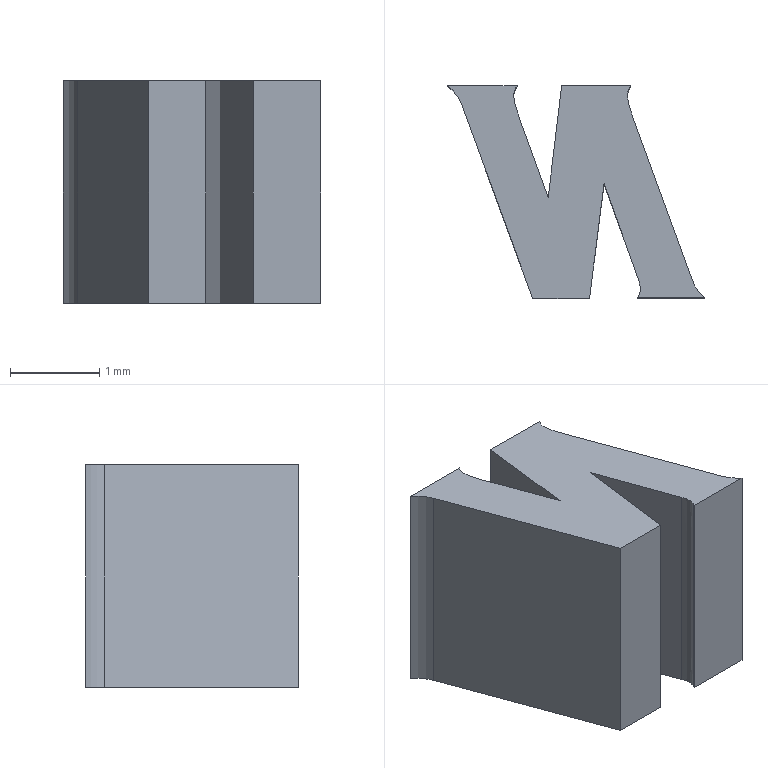Part | STEP file | lll_id1178_x_t | 1 solid | 18 faces | box 2.9 x 2.384 x 2.5 mm | volume 9.21 mm3 | plane 12 | other 4 | cylinder 2 | commonest cylinder face diameters 0.832 x1 0.919 x1
STEP:
#1=CARTESIAN_POINT('',(390.808,125.708,2.35));
#2=VERTEX_POINT('',#1);
#3=CARTESIAN_POINT('',(390.144,127.533,2.35));
#4=VERTEX_POINT('',#3);
#5=CARTESIAN_POINT('',(390.144,127.533,2.35));
#6=DIRECTION('',(-0.3422,0.9396,0.));
#7=VECTOR('',#6,1.);
#8=LINE('',#5,#7);
#9=EDGE_CURVE('',#2,#4,#8,.T.);
#10=ORIENTED_EDGE('',*,*,#9,.F.);
#11=CARTESIAN_POINT('',(390.808,125.708,-0.15));
#12=VERTEX_POINT('',#11);
#13=CARTESIAN_POINT('',(390.808,125.708,-0.15));
#14=DIRECTION('',(0.,0.,-1.));
#15=VECTOR('',#14,1.);
#16=LINE('',#13,#15);
#17=EDGE_CURVE('',#2,#12,#16,.T.);
#18=ORIENTED_EDGE('',*,*,#17,.T.);
#19=CARTESIAN_POINT('',(390.144,127.533,-0.15));
#20=VERTEX_POINT('',#19);
#21=CARTESIAN_POINT('',(390.144,127.533,-0.15));
#22=DIRECTION('',(-0.3422,0.9396,0.));
#23=VECTOR('',#22,1.);
#24=LINE('',#21,#23);
#25=EDGE_CURVE('',#12,#20,#24,.T.);
#26=ORIENTED_EDGE('',*,*,#25,.T.);
#27=CARTESIAN_POINT('',(390.144,127.533,-0.15));
#28=DIRECTION('',(0.,0.,-1.));
#29=VECTOR('',#28,1.);
#30=LINE('',#27,#29);
#31=EDGE_CURVE('',#4,#20,#30,.T.);
#32=ORIENTED_EDGE('',*,*,#31,.F.);
#33=EDGE_LOOP('',(#10,#18,#26,#32));
#34=FACE_OUTER_BOUND('',#33,.T.);
#35=CARTESIAN_POINT('',(390.144,127.533,-0.15));
#36=DIRECTION('',(-0.9396,-0.3422,0.));
#37=DIRECTION('',(-0.3422,0.9396,0.));
#38=AXIS2_PLACEMENT_3D('',#35,#36,#37);
#39=PLANE('',#38);
#40=ADVANCED_FACE('',(#34),#39,.F.);
#41=CARTESIAN_POINT('',(390.953,125.495,2.35));
#42=VERTEX_POINT('',#41);
#43=CARTESIAN_POINT('',(391.244,125.853,2.35));
#44=DIRECTION('',(0.,0.,-1.));
#45=DIRECTION('',(-1.,0.,0.));
#46=AXIS2_PLACEMENT_3D('',#43,#44,#45);
#47=CIRCLE('',#46,0.4594);
#48=EDGE_CURVE('',#42,#2,#47,.T.);
#49=ORIENTED_EDGE('',*,*,#48,.F.);
#50=CARTESIAN_POINT('',(390.953,125.495,-0.15));
#51=VERTEX_POINT('',#50);
#52=CARTESIAN_POINT('',(390.959,125.492,2.35));
#53=DIRECTION('',(0.,0.,-1.));
#54=VECTOR('',#53,1.);
#55=LINE('',#52,#54);
#56=EDGE_CURVE('',#42,#51,#55,.T.);
#57=ORIENTED_EDGE('',*,*,#56,.T.);
#58=CARTESIAN_POINT('',(391.244,125.853,-0.15));
#59=DIRECTION('',(0.,0.,-1.));
#60=DIRECTION('',(-1.,0.,0.));
#61=AXIS2_PLACEMENT_3D('',#58,#59,#60);
#62=CIRCLE('',#61,0.4594);
#63=EDGE_CURVE('',#51,#12,#62,.T.);
#64=ORIENTED_EDGE('',*,*,#63,.T.);
#65=ORIENTED_EDGE('',*,*,#17,.F.);
#66=EDGE_LOOP('',(#49,#57,#64,#65));
#67=FACE_OUTER_BOUND('',#66,.T.);
#68=CARTESIAN_POINT('',(391.244,125.853,-0.15));
#69=DIRECTION('',(0.,0.,1.));
#70=DIRECTION('',(1.,0.,0.));
#71=AXIS2_PLACEMENT_3D('',#68,#69,#70);
#72=CYLINDRICAL_SURFACE('',#71,0.4594);
#73=ADVANCED_FACE('',(#67),#72,.F.);
#74=CARTESIAN_POINT('',(390.2,125.495,2.35));
#75=VERTEX_POINT('',#74);
#76=CARTESIAN_POINT('',(390.953,125.492,2.35));
#77=DIRECTION('',(1.,0.,0.));
#78=VECTOR('',#77,1.);
#79=LINE('',#76,#78);
#80=EDGE_CURVE('',#75,#42,#79,.T.);
#81=ORIENTED_EDGE('',*,*,#80,.F.);
#82=CARTESIAN_POINT('',(390.2,125.495,-0.15));
#83=VERTEX_POINT('',#82);
#84=CARTESIAN_POINT('',(390.196,125.492,2.35));
#85=DIRECTION('',(0.,0.,-1.));
#86=VECTOR('',#85,1.);
#87=LINE('',#84,#86);
#88=EDGE_CURVE('',#75,#83,#87,.T.);
#89=ORIENTED_EDGE('',*,*,#88,.T.);
#90=CARTESIAN_POINT('',(390.953,125.492,-0.15));
#91=DIRECTION('',(1.,0.,0.));
#92=VECTOR('',#91,1.);
#93=LINE('',#90,#92);
#94=EDGE_CURVE('',#83,#51,#93,.T.);
#95=ORIENTED_EDGE('',*,*,#94,.T.);
#96=ORIENTED_EDGE('',*,*,#56,.F.);
#97=EDGE_LOOP('',(#81,#89,#95,#96));
#98=FACE_OUTER_BOUND('',#97,.T.);
#99=CARTESIAN_POINT('',(390.953,125.492,-0.15));
#100=DIRECTION('',(0.,1.,0.));
#101=DIRECTION('',(0.,0.,1.));
#102=AXIS2_PLACEMENT_3D('',#99,#100,#101);
#103=PLANE('',#102);
#104=ADVANCED_FACE('',(#98),#103,.F.);
#105=CARTESIAN_POINT('',(390.22,125.536,2.35));
#106=VERTEX_POINT('',#105);
#107=CARTESIAN_POINT('',(390.22,125.536,2.35));
#108=CARTESIAN_POINT('',(390.215,125.523,2.35));
#109=CARTESIAN_POINT('',(390.208,125.51,2.35));
#110=CARTESIAN_POINT('',(390.199,125.498,2.35));
#111=(BOUNDED_CURVE()B_SPLINE_CURVE(3,(#107,#108,#109,#110),.UNSPECIFIED.,.F.,.F.)B_SPLINE_CURVE_WITH_KNOTS((4,4),(0.,1.),.UNSPECIFIED.)CURVE()GEOMETRIC_REPRESENTATION_ITEM()RATIONAL_B_SPLINE_CURVE((0.5015,0.4995,0.4995,0.5015))REPRESENTATION_ITEM(''));
#112=EDGE_CURVE('',#106,#75,#111,.T.);
#113=ORIENTED_EDGE('',*,*,#112,.F.);
#114=CARTESIAN_POINT('',(390.22,125.536,-0.15));
#115=VERTEX_POINT('',#114);
#116=CARTESIAN_POINT('',(390.22,125.536,-0.15));
#117=DIRECTION('',(0.,0.,-1.));
#118=VECTOR('',#117,1.);
#119=LINE('',#116,#118);
#120=EDGE_CURVE('',#106,#115,#119,.T.);
#121=ORIENTED_EDGE('',*,*,#120,.T.);
#122=CARTESIAN_POINT('',(390.22,125.536,-0.15));
#123=CARTESIAN_POINT('',(390.215,125.523,-0.15));
#124=CARTESIAN_POINT('',(390.208,125.51,-0.15));
#125=CARTESIAN_POINT('',(390.199,125.497,-0.15));
#126=CARTESIAN_POINT('',(390.199,125.496,-0.15));
#127=CARTESIAN_POINT('',(390.198,125.496,-0.15));
#128=(BOUNDED_CURVE()B_SPLINE_CURVE(3,(#122,#123,#124,#125,#126,#127),.UNSPECIFIED.,.F.,.F.)B_SPLINE_CURVE_WITH_KNOTS((4,2,4),(0.,0.9573,1.),.UNSPECIFIED.)CURVE()GEOMETRIC_REPRESENTATION_ITEM()RATIONAL_B_SPLINE_CURVE((0.5015,0.4995,0.4995,0.5015,0.5015,0.5015))REPRESENTATION_ITEM(''));
#129=EDGE_CURVE('',#115,#83,#128,.T.);
#130=ORIENTED_EDGE('',*,*,#129,.T.);
#131=ORIENTED_EDGE('',*,*,#88,.F.);
#132=EDGE_LOOP('',(#113,#121,#130,#131));
#133=FACE_OUTER_BOUND('',#132,.T.);
#134=CARTESIAN_POINT('',(390.196,125.492,-0.15));
#135=CARTESIAN_POINT('',(390.196,125.493,-0.15));
#136=CARTESIAN_POINT('',(390.197,125.494,-0.15));
#137=CARTESIAN_POINT('',(390.198,125.495,-0.15));
#138=CARTESIAN_POINT('',(390.198,125.495,-0.15));
#139=CARTESIAN_POINT('',(390.199,125.496,-0.15));
#140=CARTESIAN_POINT('',(390.199,125.497,-0.15));
#141=CARTESIAN_POINT('',(390.208,125.51,-0.15));
#142=CARTESIAN_POINT('',(390.215,125.523,-0.15));
#143=CARTESIAN_POINT('',(390.22,125.536,-0.15));
#144=(BOUNDED_CURVE()B_SPLINE_CURVE(3,(#134,#135,#136,#137,#138,#139,#140,#141,#142,#143),.UNSPECIFIED.,.F.,.F.)B_SPLINE_CURVE_WITH_KNOTS((4,2,2,2,4),(0.,0.04179,0.08327,0.1224,1.),.UNSPECIFIED.)CURVE()GEOMETRIC_REPRESENTATION_ITEM()RATIONAL_B_SPLINE_CURVE((0.5015,0.5015,0.5015,0.5015,0.5015,0.5015,0.5015,0.4995,0.4995,0.5015))REPRESENTATION_ITEM(''));
#145=DIRECTION('',(0.,0.,1.));
#146=VECTOR('',#145,1.);
#147=SURFACE_OF_LINEAR_EXTRUSION('',#144,#146);
#148=ADVANCED_FACE('',(#133),#147,.F.);
#149=CARTESIAN_POINT('',(390.211,125.704,2.35));
#150=VERTEX_POINT('',#149);
#151=CARTESIAN_POINT('',(390.211,125.704,2.35));
#152=CARTESIAN_POINT('',(390.214,125.693,2.35));
#153=CARTESIAN_POINT('',(390.218,125.683,2.35));
#154=CARTESIAN_POINT('',(390.224,125.661,2.35));
#155=CARTESIAN_POINT('',(390.226,125.65,2.35));
#156=CARTESIAN_POINT('',(390.23,125.628,2.35));
#157=CARTESIAN_POINT('',(390.231,125.617,2.35));
#158=CARTESIAN_POINT('',(390.232,125.599,2.35));
#159=CARTESIAN_POINT('',(390.232,125.592,2.35));
#160=CARTESIAN_POINT('',(390.23,125.568,2.35));
#161=CARTESIAN_POINT('',(390.226,125.552,2.35));
#162=CARTESIAN_POINT('',(390.22,125.536,2.35));
#163=(BOUNDED_CURVE()B_SPLINE_CURVE(3,(#151,#152,#153,#154,#155,#156,#157,#158,#159,#160,#161,#162),.UNSPECIFIED.,.F.,.F.)B_SPLINE_CURVE_WITH_KNOTS((4,2,2,2,2,4),(0.,0.1952,0.3909,0.5862,0.7038,1.),.UNSPECIFIED.)CURVE()GEOMETRIC_REPRESENTATION_ITEM()RATIONAL_B_SPLINE_CURVE((0.5015,0.5013,0.5013,0.5011,0.5011,0.5008,0.5008,0.5011,0.5011,0.4975,0.4975,0.5015))REPRESENTATION_ITEM(''));
#164=EDGE_CURVE('',#150,#106,#163,.T.);
#165=ORIENTED_EDGE('',*,*,#164,.F.);
#166=CARTESIAN_POINT('',(390.211,125.704,-0.15));
#167=VERTEX_POINT('',#166);
#168=CARTESIAN_POINT('',(390.211,125.704,-0.15));
#169=DIRECTION('',(0.,0.,-1.));
#170=VECTOR('',#169,1.);
#171=LINE('',#168,#170);
#172=EDGE_CURVE('',#150,#167,#171,.T.);
#173=ORIENTED_EDGE('',*,*,#172,.T.);
#174=CARTESIAN_POINT('',(390.211,125.704,-0.15));
#175=CARTESIAN_POINT('',(390.214,125.693,-0.15));
#176=CARTESIAN_POINT('',(390.218,125.683,-0.15));
#177=CARTESIAN_POINT('',(390.224,125.661,-0.15));
#178=CARTESIAN_POINT('',(390.226,125.65,-0.15));
#179=CARTESIAN_POINT('',(390.23,125.628,-0.15));
#180=CARTESIAN_POINT('',(390.231,125.617,-0.15));
#181=CARTESIAN_POINT('',(390.232,125.599,-0.15));
#182=CARTESIAN_POINT('',(390.232,125.592,-0.15));
#183=CARTESIAN_POINT('',(390.23,125.568,-0.15));
#184=CARTESIAN_POINT('',(390.226,125.552,-0.15));
#185=CARTESIAN_POINT('',(390.22,125.536,-0.15));
#186=(BOUNDED_CURVE()B_SPLINE_CURVE(3,(#174,#175,#176,#177,#178,#179,#180,#181,#182,#183,#184,#185),.UNSPECIFIED.,.F.,.F.)B_SPLINE_CURVE_WITH_KNOTS((4,2,2,2,2,4),(0.,0.1952,0.3909,0.5862,0.7038,1.),.UNSPECIFIED.)CURVE()GEOMETRIC_REPRESENTATION_ITEM()RATIONAL_B_SPLINE_CURVE((0.5015,0.5013,0.5013,0.5011,0.5011,0.5008,0.5008,0.5011,0.5011,0.4975,0.4975,0.5015))REPRESENTATION_ITEM(''));
#187=EDGE_CURVE('',#167,#115,#186,.T.);
#188=ORIENTED_EDGE('',*,*,#187,.T.);
#189=ORIENTED_EDGE('',*,*,#120,.F.);
#190=EDGE_LOOP('',(#165,#173,#188,#189));
#191=FACE_OUTER_BOUND('',#190,.T.);
#192=CARTESIAN_POINT('',(390.22,125.536,-0.15));
#193=CARTESIAN_POINT('',(390.226,125.552,-0.15));
#194=CARTESIAN_POINT('',(390.23,125.568,-0.15));
#195=CARTESIAN_POINT('',(390.232,125.592,-0.15));
#196=CARTESIAN_POINT('',(390.232,125.599,-0.15));
#197=CARTESIAN_POINT('',(390.231,125.617,-0.15));
#198=CARTESIAN_POINT('',(390.23,125.628,-0.15));
#199=CARTESIAN_POINT('',(390.226,125.65,-0.15));
#200=CARTESIAN_POINT('',(390.224,125.661,-0.15));
#201=CARTESIAN_POINT('',(390.218,125.683,-0.15));
#202=CARTESIAN_POINT('',(390.214,125.693,-0.15));
#203=CARTESIAN_POINT('',(390.211,125.704,-0.15));
#204=(BOUNDED_CURVE()B_SPLINE_CURVE(3,(#192,#193,#194,#195,#196,#197,#198,#199,#200,#201,#202,#203),.UNSPECIFIED.,.F.,.F.)B_SPLINE_CURVE_WITH_KNOTS((4,2,2,2,2,4),(0.,0.2962,0.4138,0.6091,0.8048,1.),.UNSPECIFIED.)CURVE()GEOMETRIC_REPRESENTATION_ITEM()RATIONAL_B_SPLINE_CURVE((0.5015,0.4975,0.4975,0.5011,0.5011,0.5008,0.5008,0.5011,0.5011,0.5013,0.5013,0.5015))REPRESENTATION_ITEM(''));
#205=DIRECTION('',(0.,0.,1.));
#206=VECTOR('',#205,1.);
#207=SURFACE_OF_LINEAR_EXTRUSION('',#204,#206);
#208=ADVANCED_FACE('',(#191),#207,.F.);
#209=CARTESIAN_POINT('',(389.825,126.775,2.35));
#210=VERTEX_POINT('',#209);
#211=CARTESIAN_POINT('',(390.211,125.704,2.35));
#212=DIRECTION('',(0.3387,-0.9409,0.));
#213=VECTOR('',#212,1.);
#214=LINE('',#211,#213);
#215=EDGE_CURVE('',#210,#150,#214,.T.);
#216=ORIENTED_EDGE('',*,*,#215,.F.);
#217=CARTESIAN_POINT('',(389.825,126.775,-0.15));
#218=VERTEX_POINT('',#217);
#219=CARTESIAN_POINT('',(389.825,126.775,-0.15));
#220=DIRECTION('',(0.,0.,-1.));
#221=VECTOR('',#220,1.);
#222=LINE('',#219,#221);
#223=EDGE_CURVE('',#210,#218,#222,.T.);
#224=ORIENTED_EDGE('',*,*,#223,.T.);
#225=CARTESIAN_POINT('',(390.211,125.704,-0.15));
#226=DIRECTION('',(0.3387,-0.9409,0.));
#227=VECTOR('',#226,1.);
#228=LINE('',#225,#227);
#229=EDGE_CURVE('',#218,#167,#228,.T.);
#230=ORIENTED_EDGE('',*,*,#229,.T.);
#231=ORIENTED_EDGE('',*,*,#172,.F.);
#232=EDGE_LOOP('',(#216,#224,#230,#231));
#233=FACE_OUTER_BOUND('',#232,.T.);
#234=CARTESIAN_POINT('',(390.211,125.704,-0.15));
#235=DIRECTION('',(0.9409,0.3387,0.));
#236=DIRECTION('',(0.3387,-0.9409,0.));
#237=AXIS2_PLACEMENT_3D('',#234,#235,#236);
#238=PLANE('',#237);
#239=ADVANCED_FACE('',(#233),#238,.F.);
#240=CARTESIAN_POINT('',(389.662,125.492,2.35));
#241=VERTEX_POINT('',#240);
#242=CARTESIAN_POINT('',(389.825,126.775,2.35));
#243=DIRECTION('',(0.1257,0.9921,0.));
#244=VECTOR('',#243,1.);
#245=LINE('',#242,#244);
#246=EDGE_CURVE('',#241,#210,#245,.T.);
#247=ORIENTED_EDGE('',*,*,#246,.F.);
#248=CARTESIAN_POINT('',(389.662,125.492,-0.15));
#249=VERTEX_POINT('',#248);
#250=CARTESIAN_POINT('',(389.662,125.492,-0.15));
#251=DIRECTION('',(0.,0.,-1.));
#252=VECTOR('',#251,1.);
#253=LINE('',#250,#252);
#254=EDGE_CURVE('',#241,#249,#253,.T.);
#255=ORIENTED_EDGE('',*,*,#254,.T.);
#256=CARTESIAN_POINT('',(389.825,126.775,-0.15));
#257=DIRECTION('',(0.1257,0.9921,0.));
#258=VECTOR('',#257,1.);
#259=LINE('',#256,#258);
#260=EDGE_CURVE('',#249,#218,#259,.T.);
#261=ORIENTED_EDGE('',*,*,#260,.T.);
#262=ORIENTED_EDGE('',*,*,#223,.F.);
#263=EDGE_LOOP('',(#247,#255,#261,#262));
#264=FACE_OUTER_BOUND('',#263,.T.);
#265=CARTESIAN_POINT('',(389.825,126.775,-0.15));
#266=DIRECTION('',(-0.9921,0.1257,0.));
#267=DIRECTION('',(0.1257,0.9921,0.));
#268=AXIS2_PLACEMENT_3D('',#265,#266,#267);
#269=PLANE('',#268);
#270=ADVANCED_FACE('',(#264),#269,.F.);
#271=CARTESIAN_POINT('',(389.024,125.492,2.35));
#272=VERTEX_POINT('',#271);
#273=CARTESIAN_POINT('',(389.662,125.492,2.35));
#274=DIRECTION('',(1.,0.,0.));
#275=VECTOR('',#274,1.);
#276=LINE('',#273,#275);
#277=EDGE_CURVE('',#272,#241,#276,.T.);
#278=ORIENTED_EDGE('',*,*,#277,.F.);
#279=CARTESIAN_POINT('',(389.024,125.492,-0.15));
#280=VERTEX_POINT('',#279);
#281=CARTESIAN_POINT('',(389.024,125.492,-0.15));
#282=DIRECTION('',(0.,0.,-1.));
#283=VECTOR('',#282,1.);
#284=LINE('',#281,#283);
#285=EDGE_CURVE('',#272,#280,#284,.T.);
#286=ORIENTED_EDGE('',*,*,#285,.T.);
#287=CARTESIAN_POINT('',(389.662,125.492,-0.15));
#288=DIRECTION('',(1.,0.,0.));
#289=VECTOR('',#288,1.);
#290=LINE('',#287,#289);
#291=EDGE_CURVE('',#280,#249,#290,.T.);
#292=ORIENTED_EDGE('',*,*,#291,.T.);
#293=ORIENTED_EDGE('',*,*,#254,.F.);
#294=EDGE_LOOP('',(#278,#286,#292,#293));
#295=FACE_OUTER_BOUND('',#294,.T.);
#296=CARTESIAN_POINT('',(389.662,125.492,-0.15));
#297=DIRECTION('',(0.,1.,0.));
#298=DIRECTION('',(0.,0.,1.));
#299=AXIS2_PLACEMENT_3D('',#296,#297,#298);
#300=PLANE('',#299);
#301=ADVANCED_FACE('',(#295),#300,.F.);
#302=CARTESIAN_POINT('',(388.229,127.665,2.35));
#303=VERTEX_POINT('',#302);
#304=CARTESIAN_POINT('',(389.024,125.492,2.35));
#305=DIRECTION('',(0.3436,-0.9391,0.));
#306=VECTOR('',#305,1.);
#307=LINE('',#304,#306);
#308=EDGE_CURVE('',#303,#272,#307,.T.);
#309=ORIENTED_EDGE('',*,*,#308,.F.);
#310=CARTESIAN_POINT('',(388.229,127.665,-0.15));
#311=VERTEX_POINT('',#310);
#312=CARTESIAN_POINT('',(388.229,127.665,-0.15));
#313=DIRECTION('',(0.,0.,-1.));
#314=VECTOR('',#313,1.);
#315=LINE('',#312,#314);
#316=EDGE_CURVE('',#303,#311,#315,.T.);
#317=ORIENTED_EDGE('',*,*,#316,.T.);
#318=CARTESIAN_POINT('',(389.024,125.492,-0.15));
#319=DIRECTION('',(0.3436,-0.9391,0.));
#320=VECTOR('',#319,1.);
#321=LINE('',#318,#320);
#322=EDGE_CURVE('',#311,#280,#321,.T.);
#323=ORIENTED_EDGE('',*,*,#322,.T.);
#324=ORIENTED_EDGE('',*,*,#285,.F.);
#325=EDGE_LOOP('',(#309,#317,#323,#324));
#326=FACE_OUTER_BOUND('',#325,.T.);
#327=CARTESIAN_POINT('',(389.024,125.492,-0.15));
#328=DIRECTION('',(0.9391,0.3436,0.));
#329=DIRECTION('',(0.3436,-0.9391,0.));
#330=AXIS2_PLACEMENT_3D('',#327,#328,#329);
#331=PLANE('',#330);
#332=ADVANCED_FACE('',(#326),#331,.F.);
#333=CARTESIAN_POINT('',(388.068,127.874,2.35));
#334=VERTEX_POINT('',#333);
#335=CARTESIAN_POINT('',(387.837,127.525,2.35));
#336=DIRECTION('',(0.,0.,-1.));
#337=DIRECTION('',(-1.,0.,0.));
#338=AXIS2_PLACEMENT_3D('',#335,#336,#337);
#339=CIRCLE('',#338,0.4162);
#340=EDGE_CURVE('',#334,#303,#339,.T.);
#341=ORIENTED_EDGE('',*,*,#340,.F.);
#342=CARTESIAN_POINT('',(388.068,127.874,-0.15));
#343=VERTEX_POINT('',#342);
#344=CARTESIAN_POINT('',(388.059,127.877,2.35));
#345=DIRECTION('',(0.,0.,-1.));
#346=VECTOR('',#345,1.);
#347=LINE('',#344,#346);
#348=EDGE_CURVE('',#334,#343,#347,.T.);
#349=ORIENTED_EDGE('',*,*,#348,.T.);
#350=CARTESIAN_POINT('',(387.837,127.525,-0.15));
#351=DIRECTION('',(0.,0.,-1.));
#352=DIRECTION('',(-1.,0.,0.));
#353=AXIS2_PLACEMENT_3D('',#350,#351,#352);
#354=CIRCLE('',#353,0.4162);
#355=EDGE_CURVE('',#343,#311,#354,.T.);
#356=ORIENTED_EDGE('',*,*,#355,.T.);
#357=ORIENTED_EDGE('',*,*,#316,.F.);
#358=EDGE_LOOP('',(#341,#349,#356,#357));
#359=FACE_OUTER_BOUND('',#358,.T.);
#360=CARTESIAN_POINT('',(387.837,127.525,-0.15));
#361=DIRECTION('',(0.,0.,1.));
#362=DIRECTION('',(1.,0.,0.));
#363=AXIS2_PLACEMENT_3D('',#360,#361,#362);
#364=CYLINDRICAL_SURFACE('',#363,0.4162);
#365=ADVANCED_FACE('',(#359),#364,.F.);
#366=CARTESIAN_POINT('',(388.851,127.874,2.35));
#367=VERTEX_POINT('',#366);
#368=CARTESIAN_POINT('',(388.068,127.877,2.35));
#369=DIRECTION('',(-1.,0.,0.));
#370=VECTOR('',#369,1.);
#371=LINE('',#368,#370);
#372=EDGE_CURVE('',#367,#334,#371,.T.);
#373=ORIENTED_EDGE('',*,*,#372,.F.);
#374=CARTESIAN_POINT('',(388.851,127.874,-0.15));
#375=VERTEX_POINT('',#374);
#376=CARTESIAN_POINT('',(388.855,127.877,2.35));
#377=DIRECTION('',(0.,0.,-1.));
#378=VECTOR('',#377,1.);
#379=LINE('',#376,#378);
#380=EDGE_CURVE('',#367,#375,#379,.T.);
#381=ORIENTED_EDGE('',*,*,#380,.T.);
#382=CARTESIAN_POINT('',(388.068,127.877,-0.15));
#383=DIRECTION('',(-1.,0.,0.));
#384=VECTOR('',#383,1.);
#385=LINE('',#382,#384);
#386=EDGE_CURVE('',#375,#343,#385,.T.);
#387=ORIENTED_EDGE('',*,*,#386,.T.);
#388=ORIENTED_EDGE('',*,*,#348,.F.);
#389=EDGE_LOOP('',(#373,#381,#387,#388));
#390=FACE_OUTER_BOUND('',#389,.T.);
#391=CARTESIAN_POINT('',(388.068,127.877,-0.15));
#392=DIRECTION('',(0.,-1.,0.));
#393=DIRECTION('',(0.,0.,-1.));
#394=AXIS2_PLACEMENT_3D('',#391,#392,#393);
#395=PLANE('',#394);
#396=ADVANCED_FACE('',(#390),#395,.F.);
#397=CARTESIAN_POINT('',(388.868,127.533,2.35));
#398=VERTEX_POINT('',#397);
#399=CARTESIAN_POINT('',(388.868,127.533,2.35));
#400=CARTESIAN_POINT('',(388.86,127.554,2.35));
#401=CARTESIAN_POINT('',(388.853,127.575,2.35));
#402=CARTESIAN_POINT('',(388.841,127.614,2.35));
#403=CARTESIAN_POINT('',(388.836,127.631,2.35));
#404=CARTESIAN_POINT('',(388.827,127.66,2.35));
#405=CARTESIAN_POINT('',(388.825,127.671,2.35));
#406=CARTESIAN_POINT('',(388.819,127.692,2.35));
#407=CARTESIAN_POINT('',(388.817,127.703,2.35));
#408=CARTESIAN_POINT('',(388.814,127.723,2.35));
#409=CARTESIAN_POINT('',(388.813,127.733,2.35));
#410=CARTESIAN_POINT('',(388.811,127.755,2.35));
#411=CARTESIAN_POINT('',(388.811,127.768,2.35));
#412=CARTESIAN_POINT('',(388.815,127.81,2.35));
#413=CARTESIAN_POINT('',(388.826,127.839,2.35));
#414=CARTESIAN_POINT('',(388.846,127.865,2.35));
#415=CARTESIAN_POINT('',(388.849,127.868,2.35));
#416=CARTESIAN_POINT('',(388.851,127.871,2.35));
#417=(BOUNDED_CURVE()B_SPLINE_CURVE(3,(#399,#400,#401,#402,#403,#404,#405,#406,#407,#408,#409,#410,#411,#412,#413,#414,#415,#416),.UNSPECIFIED.,.F.,.F.)B_SPLINE_CURVE_WITH_KNOTS((4,2,2,2,2,2,2,2,4),(0.,0.1864,0.3417,0.4351,0.5283,0.6059,0.715,0.9678,1.),.UNSPECIFIED.)CURVE()GEOMETRIC_REPRESENTATION_ITEM()RATIONAL_B_SPLINE_CURVE((0.5001,0.5,0.5,0.5,0.5,0.5,0.5,0.4998,0.4998,0.4998,0.4998,0.4988,0.4988,0.4872,0.4872,0.5,0.5,0.5001))REPRESENTATION_ITEM(''));
#418=EDGE_CURVE('',#398,#367,#417,.T.);
#419=ORIENTED_EDGE('',*,*,#418,.F.);
#420=CARTESIAN_POINT('',(388.868,127.533,-0.15));
#421=VERTEX_POINT('',#420);
#422=CARTESIAN_POINT('',(388.868,127.533,-0.15));
#423=DIRECTION('',(0.,0.,-1.));
#424=VECTOR('',#423,1.);
#425=LINE('',#422,#424);
#426=EDGE_CURVE('',#398,#421,#425,.T.);
#427=ORIENTED_EDGE('',*,*,#426,.T.);
#428=CARTESIAN_POINT('',(388.868,127.533,-0.15));
#429=CARTESIAN_POINT('',(388.86,127.554,-0.15));
#430=CARTESIAN_POINT('',(388.853,127.575,-0.15));
#431=CARTESIAN_POINT('',(388.841,127.614,-0.15));
#432=CARTESIAN_POINT('',(388.836,127.631,-0.15));
#433=CARTESIAN_POINT('',(388.827,127.66,-0.15));
#434=CARTESIAN_POINT('',(388.825,127.671,-0.15));
#435=CARTESIAN_POINT('',(388.819,127.692,-0.15));
#436=CARTESIAN_POINT('',(388.817,127.703,-0.15));
#437=CARTESIAN_POINT('',(388.814,127.723,-0.15));
#438=CARTESIAN_POINT('',(388.813,127.733,-0.15));
#439=CARTESIAN_POINT('',(388.811,127.755,-0.15));
#440=CARTESIAN_POINT('',(388.811,127.768,-0.15));
#441=CARTESIAN_POINT('',(388.815,127.81,-0.15));
#442=CARTESIAN_POINT('',(388.826,127.839,-0.15));
#443=CARTESIAN_POINT('',(388.846,127.865,-0.15));
#444=CARTESIAN_POINT('',(388.849,127.868,-0.15));
#445=CARTESIAN_POINT('',(388.852,127.872,-0.15));
#446=CARTESIAN_POINT('',(388.852,127.873,-0.15));
#447=CARTESIAN_POINT('',(388.853,127.874,-0.15));
#448=(BOUNDED_CURVE()B_SPLINE_CURVE(3,(#428,#429,#430,#431,#432,#433,#434,#435,#436,#437,#438,#439,#440,#441,#442,#443,#444,#445,#446,#447),.UNSPECIFIED.,.F.,.F.)B_SPLINE_CURVE_WITH_KNOTS((4,2,2,2,2,2,2,2,2,4),(0.,0.1846,0.3383,0.4308,0.5231,0.5999,0.7079,0.9582,0.9901,1.),.UNSPECIFIED.)CURVE()GEOMETRIC_REPRESENTATION_ITEM()RATIONAL_B_SPLINE_CURVE((0.5001,0.5,0.5,0.5,0.5,0.5,0.5,0.4998,0.4998,0.4998,0.4998,0.4988,0.4988,0.4872,0.4872,0.5,0.5,0.5001,0.5001,0.5001))REPRESENTATION_ITEM(''));
#449=EDGE_CURVE('',#421,#375,#448,.T.);
#450=ORIENTED_EDGE('',*,*,#449,.T.);
#451=ORIENTED_EDGE('',*,*,#380,.F.);
#452=EDGE_LOOP('',(#419,#427,#450,#451));
#453=FACE_OUTER_BOUND('',#452,.T.);
#454=CARTESIAN_POINT('',(388.858,127.879,-0.15));
#455=CARTESIAN_POINT('',(388.857,127.878,-0.15));
#456=CARTESIAN_POINT('',(388.856,127.877,-0.15));
#457=CARTESIAN_POINT('',(388.855,127.876,-0.15));
#458=CARTESIAN_POINT('',(388.854,127.875,-0.15));
#459=CARTESIAN_POINT('',(388.852,127.873,-0.15));
#460=CARTESIAN_POINT('',(388.852,127.872,-0.15));
#461=CARTESIAN_POINT('',(388.849,127.868,-0.15));
#462=CARTESIAN_POINT('',(388.846,127.865,-0.15));
#463=CARTESIAN_POINT('',(388.826,127.839,-0.15));
#464=CARTESIAN_POINT('',(388.815,127.81,-0.15));
#465=CARTESIAN_POINT('',(388.811,127.768,-0.15));
#466=CARTESIAN_POINT('',(388.811,127.755,-0.15));
#467=CARTESIAN_POINT('',(388.813,127.733,-0.15));
#468=CARTESIAN_POINT('',(388.814,127.723,-0.15));
#469=CARTESIAN_POINT('',(388.817,127.703,-0.15));
#470=CARTESIAN_POINT('',(388.819,127.692,-0.15));
#471=CARTESIAN_POINT('',(388.825,127.671,-0.15));
#472=CARTESIAN_POINT('',(388.827,127.66,-0.15));
#473=CARTESIAN_POINT('',(388.836,127.631,-0.15));
#474=CARTESIAN_POINT('',(388.841,127.614,-0.15));
#475=CARTESIAN_POINT('',(388.853,127.575,-0.15));
#476=CARTESIAN_POINT('',(388.86,127.554,-0.15));
#477=CARTESIAN_POINT('',(388.868,127.533,-0.15));
#478=(BOUNDED_CURVE()B_SPLINE_CURVE(3,(#454,#455,#456,#457,#458,#459,#460,#461,#462,#463,#464,#465,#466,#467,#468,#469,#470,#471,#472,#473,#474,#475,#476,#477),.UNSPECIFIED.,.F.,.F.)B_SPLINE_CURVE_WITH_KNOTS((4,2,2,2,2,2,2,2,2,2,2,4),(0.,0.009901,0.0197,0.02941,0.06067,0.306,0.4119,0.4872,0.5777,0.6684,0.8191,1.),.UNSPECIFIED.)CURVE()GEOMETRIC_REPRESENTATION_ITEM()RATIONAL_B_SPLINE_CURVE((0.5001,0.5001,0.5001,0.5001,0.5001,0.5001,0.5001,0.5,0.5,0.4872,0.4872,0.4988,0.4988,0.4998,0.4998,0.4998,0.4998,0.5,0.5,0.5,0.5,0.5,0.5,0.5001))REPRESENTATION_ITEM(''));
#479=DIRECTION('',(0.,0.,1.));
#480=VECTOR('',#479,1.);
#481=SURFACE_OF_LINEAR_EXTRUSION('',#478,#480);
#482=ADVANCED_FACE('',(#453),#481,.F.);
#483=CARTESIAN_POINT('',(389.199,126.625,2.35));
#484=VERTEX_POINT('',#483);
#485=CARTESIAN_POINT('',(388.868,127.533,2.35));
#486=DIRECTION('',(-0.3421,0.9397,0.));
#487=VECTOR('',#486,1.);
#488=LINE('',#485,#487);
#489=EDGE_CURVE('',#484,#398,#488,.T.);
#490=ORIENTED_EDGE('',*,*,#489,.F.);
#491=CARTESIAN_POINT('',(389.199,126.625,-0.15));
#492=VERTEX_POINT('',#491);
#493=CARTESIAN_POINT('',(389.199,126.625,-0.15));
#494=DIRECTION('',(0.,0.,-1.));
#495=VECTOR('',#494,1.);
#496=LINE('',#493,#495);
#497=EDGE_CURVE('',#484,#492,#496,.T.);
#498=ORIENTED_EDGE('',*,*,#497,.T.);
#499=CARTESIAN_POINT('',(388.868,127.533,-0.15));
#500=DIRECTION('',(-0.3421,0.9397,0.));
#501=VECTOR('',#500,1.);
#502=LINE('',#499,#501);
#503=EDGE_CURVE('',#492,#421,#502,.T.);
#504=ORIENTED_EDGE('',*,*,#503,.T.);
#505=ORIENTED_EDGE('',*,*,#426,.F.);
#506=EDGE_LOOP('',(#490,#498,#504,#505));
#507=FACE_OUTER_BOUND('',#506,.T.);
#508=CARTESIAN_POINT('',(388.868,127.533,-0.15));
#509=DIRECTION('',(-0.9397,-0.3421,0.));
#510=DIRECTION('',(-0.3421,0.9397,0.));
#511=AXIS2_PLACEMENT_3D('',#508,#509,#510);
#512=PLANE('',#511);
#513=ADVANCED_FACE('',(#507),#512,.F.);
#514=CARTESIAN_POINT('',(389.35,127.877,2.35));
#515=VERTEX_POINT('',#514);
#516=CARTESIAN_POINT('',(389.199,126.625,2.35));
#517=DIRECTION('',(-0.1198,-0.9928,0.));
#518=VECTOR('',#517,1.);
#519=LINE('',#516,#518);
#520=EDGE_CURVE('',#515,#484,#519,.T.);
#521=ORIENTED_EDGE('',*,*,#520,.F.);
#522=CARTESIAN_POINT('',(389.35,127.877,-0.15));
#523=VERTEX_POINT('',#522);
#524=CARTESIAN_POINT('',(389.35,127.877,-0.15));
#525=DIRECTION('',(0.,0.,-1.));
#526=VECTOR('',#525,1.);
#527=LINE('',#524,#526);
#528=EDGE_CURVE('',#515,#523,#527,.T.);
#529=ORIENTED_EDGE('',*,*,#528,.T.);
#530=CARTESIAN_POINT('',(389.199,126.625,-0.15));
#531=DIRECTION('',(-0.1198,-0.9928,0.));
#532=VECTOR('',#531,1.);
#533=LINE('',#530,#532);
#534=EDGE_CURVE('',#523,#492,#533,.T.);
#535=ORIENTED_EDGE('',*,*,#534,.T.);
#536=ORIENTED_EDGE('',*,*,#497,.F.);
#537=EDGE_LOOP('',(#521,#529,#535,#536));
#538=FACE_OUTER_BOUND('',#537,.T.);
#539=CARTESIAN_POINT('',(389.199,126.625,-0.15));
#540=DIRECTION('',(0.9928,-0.1198,0.));
#541=DIRECTION('',(-0.1198,-0.9928,0.));
#542=AXIS2_PLACEMENT_3D('',#539,#540,#541);
#543=PLANE('',#542);
#544=ADVANCED_FACE('',(#538),#543,.F.);
#545=CARTESIAN_POINT('',(390.126,127.874,2.35));
#546=VERTEX_POINT('',#545);
#547=CARTESIAN_POINT('',(389.35,127.877,2.35));
#548=DIRECTION('',(-1.,0.,0.));
#549=VECTOR('',#548,1.);
#550=LINE('',#547,#549);
#551=EDGE_CURVE('',#546,#515,#550,.T.);
#552=ORIENTED_EDGE('',*,*,#551,.F.);
#553=CARTESIAN_POINT('',(390.126,127.874,-0.15));
#554=VERTEX_POINT('',#553);
#555=CARTESIAN_POINT('',(390.131,127.877,2.35));
#556=DIRECTION('',(0.,0.,-1.));
#557=VECTOR('',#556,1.);
#558=LINE('',#555,#557);
#559=EDGE_CURVE('',#546,#554,#558,.T.);
#560=ORIENTED_EDGE('',*,*,#559,.T.);
#561=CARTESIAN_POINT('',(389.35,127.877,-0.15));
#562=DIRECTION('',(-1.,0.,0.));
#563=VECTOR('',#562,1.);
#564=LINE('',#561,#563);
#565=EDGE_CURVE('',#554,#523,#564,.T.);
#566=ORIENTED_EDGE('',*,*,#565,.T.);
#567=ORIENTED_EDGE('',*,*,#528,.F.);
#568=EDGE_LOOP('',(#552,#560,#566,#567));
#569=FACE_OUTER_BOUND('',#568,.T.);
#570=CARTESIAN_POINT('',(389.35,127.877,-0.15));
#571=DIRECTION('',(0.,-1.,0.));
#572=DIRECTION('',(0.,0.,-1.));
#573=AXIS2_PLACEMENT_3D('',#570,#571,#572);
#574=PLANE('',#573);
#575=ADVANCED_FACE('',(#569),#574,.F.);
#576=CARTESIAN_POINT('',(390.144,127.533,2.35));
#577=CARTESIAN_POINT('',(390.136,127.554,2.35));
#578=CARTESIAN_POINT('',(390.129,127.575,2.35));
#579=CARTESIAN_POINT('',(390.117,127.614,2.35));
#580=CARTESIAN_POINT('',(390.111,127.632,2.35));
#581=CARTESIAN_POINT('',(390.103,127.66,2.35));
#582=CARTESIAN_POINT('',(390.1,127.671,2.35));
#583=CARTESIAN_POINT('',(390.095,127.692,2.35));
#584=CARTESIAN_POINT('',(390.093,127.703,2.35));
#585=CARTESIAN_POINT('',(390.089,127.725,2.35));
#586=CARTESIAN_POINT('',(390.088,127.736,2.35));
#587=CARTESIAN_POINT('',(390.087,127.76,2.35));
#588=CARTESIAN_POINT('',(390.087,127.773,2.35));
#589=CARTESIAN_POINT('',(390.092,127.814,2.35));
#590=CARTESIAN_POINT('',(390.102,127.84,2.35));
#591=CARTESIAN_POINT('',(390.122,127.865,2.35));
#592=CARTESIAN_POINT('',(390.124,127.868,2.35));
#593=CARTESIAN_POINT('',(390.126,127.871,2.35));
#594=(BOUNDED_CURVE()B_SPLINE_CURVE(3,(#576,#577,#578,#579,#580,#581,#582,#583,#584,#585,#586,#587,#588,#589,#590,#591,#592,#593),.UNSPECIFIED.,.F.,.F.)B_SPLINE_CURVE_WITH_KNOTS((4,2,2,2,2,2,2,2,4),(0.,0.1865,0.3418,0.4353,0.5286,0.6217,0.731,0.9679,1.),.UNSPECIFIED.)CURVE()GEOMETRIC_REPRESENTATION_ITEM()RATIONAL_B_SPLINE_CURVE((0.5001,0.5,0.5,0.5001,0.5001,0.5,0.5,0.4998,0.4998,0.4996,0.4996,0.4987,0.4987,0.4886,0.4886,0.5,0.5,0.5001))REPRESENTATION_ITEM(''));
#595=EDGE_CURVE('',#4,#546,#594,.T.);
#596=ORIENTED_EDGE('',*,*,#595,.F.);
#597=ORIENTED_EDGE('',*,*,#31,.T.);
#598=CARTESIAN_POINT('',(390.144,127.533,-0.15));
#599=CARTESIAN_POINT('',(390.136,127.554,-0.15));
#600=CARTESIAN_POINT('',(390.129,127.575,-0.15));
#601=CARTESIAN_POINT('',(390.117,127.614,-0.15));
#602=CARTESIAN_POINT('',(390.111,127.632,-0.15));
#603=CARTESIAN_POINT('',(390.103,127.66,-0.15));
#604=CARTESIAN_POINT('',(390.1,127.671,-0.15));
#605=CARTESIAN_POINT('',(390.095,127.692,-0.15));
#606=CARTESIAN_POINT('',(390.093,127.703,-0.15));
#607=CARTESIAN_POINT('',(390.089,127.725,-0.15));
#608=CARTESIAN_POINT('',(390.088,127.736,-0.15));
#609=CARTESIAN_POINT('',(390.087,127.76,-0.15));
#610=CARTESIAN_POINT('',(390.087,127.773,-0.15));
#611=CARTESIAN_POINT('',(390.092,127.814,-0.15));
#612=CARTESIAN_POINT('',(390.102,127.84,-0.15));
#613=CARTESIAN_POINT('',(390.122,127.865,-0.15));
#614=CARTESIAN_POINT('',(390.124,127.868,-0.15));
#615=CARTESIAN_POINT('',(390.127,127.872,-0.15));
#616=CARTESIAN_POINT('',(390.128,127.873,-0.15));
#617=CARTESIAN_POINT('',(390.129,127.874,-0.15));
#618=(BOUNDED_CURVE()B_SPLINE_CURVE(3,(#598,#599,#600,#601,#602,#603,#604,#605,#606,#607,#608,#609,#610,#611,#612,#613,#614,#615,#616,#617),.UNSPECIFIED.,.F.,.F.)B_SPLINE_CURVE_WITH_KNOTS((4,2,2,2,2,2,2,2,2,4),(0.,0.1847,0.3385,0.431,0.5234,0.6156,0.7238,0.9583,0.9901,1.),.UNSPECIFIED.)CURVE()GEOMETRIC_REPRESENTATION_ITEM()RATIONAL_B_SPLINE_CURVE((0.5001,0.5,0.5,0.5001,0.5001,0.5,0.5,0.4998,0.4998,0.4996,0.4996,0.4987,0.4987,0.4886,0.4886,0.5,0.5,0.5001,0.5001,0.5001))REPRESENTATION_ITEM(''));
#619=EDGE_CURVE('',#20,#554,#618,.T.);
#620=ORIENTED_EDGE('',*,*,#619,.T.);
#621=ORIENTED_EDGE('',*,*,#559,.F.);
#622=EDGE_LOOP('',(#596,#597,#620,#621));
#623=FACE_OUTER_BOUND('',#622,.T.);
#624=CARTESIAN_POINT('',(390.133,127.879,-0.15));
#625=CARTESIAN_POINT('',(390.132,127.878,-0.15));
#626=CARTESIAN_POINT('',(390.132,127.877,-0.15));
#627=CARTESIAN_POINT('',(390.13,127.876,-0.15));
#628=CARTESIAN_POINT('',(390.129,127.875,-0.15));
#629=CARTESIAN_POINT('',(390.128,127.873,-0.15));
#630=CARTESIAN_POINT('',(390.127,127.872,-0.15));
#631=CARTESIAN_POINT('',(390.124,127.868,-0.15));
#632=CARTESIAN_POINT('',(390.122,127.865,-0.15));
#633=CARTESIAN_POINT('',(390.102,127.84,-0.15));
#634=CARTESIAN_POINT('',(390.092,127.814,-0.15));
#635=CARTESIAN_POINT('',(390.087,127.773,-0.15));
#636=CARTESIAN_POINT('',(390.087,127.76,-0.15));
#637=CARTESIAN_POINT('',(390.088,127.736,-0.15));
#638=CARTESIAN_POINT('',(390.089,127.725,-0.15));
#639=CARTESIAN_POINT('',(390.093,127.703,-0.15));
#640=CARTESIAN_POINT('',(390.095,127.692,-0.15));
#641=CARTESIAN_POINT('',(390.1,127.671,-0.15));
#642=CARTESIAN_POINT('',(390.103,127.66,-0.15));
#643=CARTESIAN_POINT('',(390.111,127.632,-0.15));
#644=CARTESIAN_POINT('',(390.117,127.614,-0.15));
#645=CARTESIAN_POINT('',(390.129,127.575,-0.15));
#646=CARTESIAN_POINT('',(390.136,127.554,-0.15));
#647=CARTESIAN_POINT('',(390.144,127.533,-0.15));
#648=(BOUNDED_CURVE()B_SPLINE_CURVE(3,(#624,#625,#626,#627,#628,#629,#630,#631,#632,#633,#634,#635,#636,#637,#638,#639,#640,#641,#642,#643,#644,#645,#646,#647),.UNSPECIFIED.,.F.,.F.)B_SPLINE_CURVE_WITH_KNOTS((4,2,2,2,2,2,2,2,2,2,2,4),(0.,0.009901,0.0197,0.02941,0.06061,0.2905,0.3966,0.4869,0.5775,0.6682,0.819,1.),.UNSPECIFIED.)CURVE()GEOMETRIC_REPRESENTATION_ITEM()RATIONAL_B_SPLINE_CURVE((0.5001,0.5001,0.5001,0.5001,0.5001,0.5001,0.5001,0.5,0.5,0.4886,0.4886,0.4987,0.4987,0.4996,0.4996,0.4998,0.4998,0.5,0.5,0.5001,0.5001,0.5,0.5,0.5001))REPRESENTATION_ITEM(''));
#649=DIRECTION('',(0.,0.,1.));
#650=VECTOR('',#649,1.);
#651=SURFACE_OF_LINEAR_EXTRUSION('',#648,#650);
#652=ADVANCED_FACE('',(#623),#651,.F.);
#653=ORIENTED_EDGE('',*,*,#25,.F.);
#654=ORIENTED_EDGE('',*,*,#63,.F.);
#655=ORIENTED_EDGE('',*,*,#94,.F.);
#656=ORIENTED_EDGE('',*,*,#129,.F.);
#657=ORIENTED_EDGE('',*,*,#187,.F.);
#658=ORIENTED_EDGE('',*,*,#229,.F.);
#659=ORIENTED_EDGE('',*,*,#260,.F.);
#660=ORIENTED_EDGE('',*,*,#291,.F.);
#661=ORIENTED_EDGE('',*,*,#322,.F.);
#662=ORIENTED_EDGE('',*,*,#355,.F.);
#663=ORIENTED_EDGE('',*,*,#386,.F.);
#664=ORIENTED_EDGE('',*,*,#449,.F.);
#665=ORIENTED_EDGE('',*,*,#503,.F.);
#666=ORIENTED_EDGE('',*,*,#534,.F.);
#667=ORIENTED_EDGE('',*,*,#565,.F.);
#668=ORIENTED_EDGE('',*,*,#619,.F.);
#669=EDGE_LOOP('',(#653,#654,#655,#656,#657,#658,#659,#660,#661,#662,#663,#664,#665,#666,#667,#668));
#670=FACE_OUTER_BOUND('',#669,.T.);
#671=CARTESIAN_POINT('',(391.244,125.853,-0.15));
#672=DIRECTION('',(0.,0.,1.));
#673=DIRECTION('',(1.,0.,0.));
#674=AXIS2_PLACEMENT_3D('',#671,#672,#673);
#675=PLANE('',#674);
#676=ADVANCED_FACE('',(#670),#675,.F.);
#677=ORIENTED_EDGE('',*,*,#9,.T.);
#678=ORIENTED_EDGE('',*,*,#595,.T.);
#679=ORIENTED_EDGE('',*,*,#551,.T.);
#680=ORIENTED_EDGE('',*,*,#520,.T.);
#681=ORIENTED_EDGE('',*,*,#489,.T.);
#682=ORIENTED_EDGE('',*,*,#418,.T.);
#683=ORIENTED_EDGE('',*,*,#372,.T.);
#684=ORIENTED_EDGE('',*,*,#340,.T.);
#685=ORIENTED_EDGE('',*,*,#308,.T.);
#686=ORIENTED_EDGE('',*,*,#277,.T.);
#687=ORIENTED_EDGE('',*,*,#246,.T.);
#688=ORIENTED_EDGE('',*,*,#215,.T.);
#689=ORIENTED_EDGE('',*,*,#164,.T.);
#690=ORIENTED_EDGE('',*,*,#112,.T.);
#691=ORIENTED_EDGE('',*,*,#80,.T.);
#692=ORIENTED_EDGE('',*,*,#48,.T.);
#693=EDGE_LOOP('',(#677,#678,#679,#680,#681,#682,#683,#684,#685,#686,#687,#688,#689,#690,#691,#692));
#694=FACE_OUTER_BOUND('',#693,.T.);
#695=CARTESIAN_POINT('',(391.244,125.853,2.35));
#696=DIRECTION('',(0.,0.,1.));
#697=DIRECTION('',(1.,0.,0.));
#698=AXIS2_PLACEMENT_3D('',#695,#696,#697);
#699=PLANE('',#698);
#700=ADVANCED_FACE('',(#694),#699,.T.);
#701=CLOSED_SHELL('',(#40,#73,#104,#148,#208,#239,#270,#301,#332,#365,#396,#482,#513,#544,#575,#652,#676,#700));
#702=MANIFOLD_SOLID_BREP('',#701);
#703=(LENGTH_UNIT()NAMED_UNIT(*)SI_UNIT(.MILLI.,.METRE.));
#704=UNCERTAINTY_MEASURE_WITH_UNIT(LENGTH_MEASURE(0.01816),#703,'','');
#705=(NAMED_UNIT(*)PLANE_ANGLE_UNIT()SI_UNIT($,.RADIAN.));
#706=PLANE_ANGLE_MEASURE_WITH_UNIT(PLANE_ANGLE_MEASURE(0.01745),#705);
#707=DIMENSIONAL_EXPONENTS(0.,0.,0.,0.,0.,0.,0.);
#708=(CONVERSION_BASED_UNIT('DEGREE',#706)NAMED_UNIT(#707)PLANE_ANGLE_UNIT());
#709=(NAMED_UNIT(*)SI_UNIT($,.STERADIAN.)SOLID_ANGLE_UNIT());
#710=(GEOMETRIC_REPRESENTATION_CONTEXT(3)GLOBAL_UNCERTAINTY_ASSIGNED_CONTEXT((#704))GLOBAL_UNIT_ASSIGNED_CONTEXT((#703,#708,#709))REPRESENTATION_CONTEXT('',''));
#711=ADVANCED_BREP_SHAPE_REPRESENTATION('',(#702),#710);